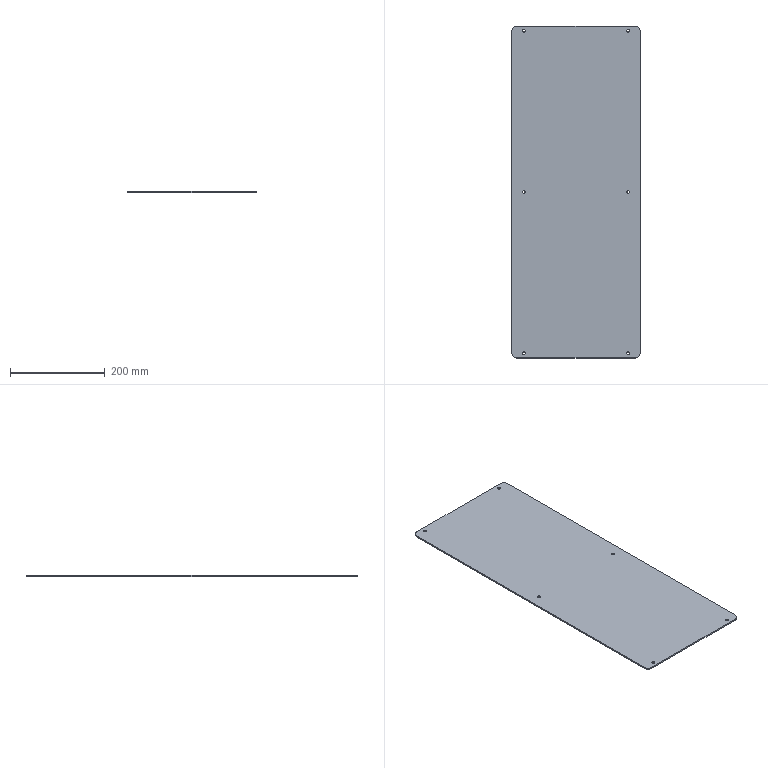Part | STEP file | 09-13 light-transmitting plate | 1 solid | 22 faces | box 270 x 700 x 3 mm | volume 566234 mm3 | cylinder 16 | plane 6 | commonest cylinder face diameters 6 x12 20 x4
STEP:
#1=CARTESIAN_POINT('',(107.,-340.,3.));
#2=VERTEX_POINT('',#1);
#3=CARTESIAN_POINT('',(113.,-340.,3.));
#4=VERTEX_POINT('',#3);
#5=CARTESIAN_POINT('',(110.,-340.,3.));
#6=DIRECTION('',(0.,0.,1.));
#7=DIRECTION('',(1.,0.,0.));
#8=AXIS2_PLACEMENT_3D('',#5,#6,#7);
#9=CIRCLE('',#8,3.);
#10=EDGE_CURVE('',#2,#4,#9,.T.);
#11=ORIENTED_EDGE('',*,*,#10,.T.);
#12=CARTESIAN_POINT('',(113.,-340.,0.));
#13=VERTEX_POINT('',#12);
#14=CARTESIAN_POINT('',(113.,-340.,6.));
#15=DIRECTION('',(0.,0.,-1.));
#16=VECTOR('',#15,1000.);
#17=LINE('',#14,#16);
#18=EDGE_CURVE('',#4,#13,#17,.T.);
#19=ORIENTED_EDGE('',*,*,#18,.T.);
#20=CARTESIAN_POINT('',(107.,-340.,0.));
#21=VERTEX_POINT('',#20);
#22=CARTESIAN_POINT('',(110.,-340.,0.));
#23=DIRECTION('',(0.,0.,-1.));
#24=DIRECTION('',(-1.,0.,0.));
#25=AXIS2_PLACEMENT_3D('',#22,#23,#24);
#26=CIRCLE('',#25,3.);
#27=EDGE_CURVE('',#13,#21,#26,.T.);
#28=ORIENTED_EDGE('',*,*,#27,.T.);
#29=CARTESIAN_POINT('',(107.,-340.,6.));
#30=DIRECTION('',(0.,0.,-1.));
#31=VECTOR('',#30,1000.);
#32=LINE('',#29,#31);
#33=EDGE_CURVE('',#2,#21,#32,.T.);
#34=ORIENTED_EDGE('',*,*,#33,.F.);
#35=EDGE_LOOP('',(#11,#19,#28,#34));
#36=FACE_OUTER_BOUND('',#35,.T.);
#37=CARTESIAN_POINT('',(110.,-340.,6.));
#38=DIRECTION('',(0.,0.,-1.));
#39=DIRECTION('',(-1.,0.,0.));
#40=AXIS2_PLACEMENT_3D('',#37,#38,#39);
#41=CYLINDRICAL_SURFACE('',#40,3.);
#42=ADVANCED_FACE('',(#36),#41,.F.);
#43=CARTESIAN_POINT('',(107.,0.,3.));
#44=VERTEX_POINT('',#43);
#45=CARTESIAN_POINT('',(113.,0.,3.));
#46=VERTEX_POINT('',#45);
#47=CARTESIAN_POINT('',(110.,0.,3.));
#48=DIRECTION('',(0.,0.,1.));
#49=DIRECTION('',(1.,0.,0.));
#50=AXIS2_PLACEMENT_3D('',#47,#48,#49);
#51=CIRCLE('',#50,3.);
#52=EDGE_CURVE('',#44,#46,#51,.T.);
#53=ORIENTED_EDGE('',*,*,#52,.T.);
#54=CARTESIAN_POINT('',(113.,0.,0.));
#55=VERTEX_POINT('',#54);
#56=CARTESIAN_POINT('',(113.,0.,6.));
#57=DIRECTION('',(0.,0.,-1.));
#58=VECTOR('',#57,1000.);
#59=LINE('',#56,#58);
#60=EDGE_CURVE('',#46,#55,#59,.T.);
#61=ORIENTED_EDGE('',*,*,#60,.T.);
#62=CARTESIAN_POINT('',(107.,0.,0.));
#63=VERTEX_POINT('',#62);
#64=CARTESIAN_POINT('',(110.,0.,0.));
#65=DIRECTION('',(0.,0.,-1.));
#66=DIRECTION('',(-1.,0.,0.));
#67=AXIS2_PLACEMENT_3D('',#64,#65,#66);
#68=CIRCLE('',#67,3.);
#69=EDGE_CURVE('',#55,#63,#68,.T.);
#70=ORIENTED_EDGE('',*,*,#69,.T.);
#71=CARTESIAN_POINT('',(107.,0.,6.));
#72=DIRECTION('',(0.,0.,-1.));
#73=VECTOR('',#72,1000.);
#74=LINE('',#71,#73);
#75=EDGE_CURVE('',#44,#63,#74,.T.);
#76=ORIENTED_EDGE('',*,*,#75,.F.);
#77=EDGE_LOOP('',(#53,#61,#70,#76));
#78=FACE_OUTER_BOUND('',#77,.T.);
#79=CARTESIAN_POINT('',(110.,0.,6.));
#80=DIRECTION('',(0.,0.,-1.));
#81=DIRECTION('',(-1.,0.,0.));
#82=AXIS2_PLACEMENT_3D('',#79,#80,#81);
#83=CYLINDRICAL_SURFACE('',#82,3.);
#84=ADVANCED_FACE('',(#78),#83,.F.);
#85=CARTESIAN_POINT('',(-113.,-340.,3.));
#86=VERTEX_POINT('',#85);
#87=CARTESIAN_POINT('',(-107.,-340.,3.));
#88=VERTEX_POINT('',#87);
#89=CARTESIAN_POINT('',(-110.,-340.,3.));
#90=DIRECTION('',(0.,0.,1.));
#91=DIRECTION('',(1.,0.,0.));
#92=AXIS2_PLACEMENT_3D('',#89,#90,#91);
#93=CIRCLE('',#92,3.);
#94=EDGE_CURVE('',#86,#88,#93,.T.);
#95=ORIENTED_EDGE('',*,*,#94,.T.);
#96=CARTESIAN_POINT('',(-107.,-340.,0.));
#97=VERTEX_POINT('',#96);
#98=CARTESIAN_POINT('',(-107.,-340.,6.));
#99=DIRECTION('',(0.,0.,-1.));
#100=VECTOR('',#99,1000.);
#101=LINE('',#98,#100);
#102=EDGE_CURVE('',#88,#97,#101,.T.);
#103=ORIENTED_EDGE('',*,*,#102,.T.);
#104=CARTESIAN_POINT('',(-113.,-340.,0.));
#105=VERTEX_POINT('',#104);
#106=CARTESIAN_POINT('',(-110.,-340.,0.));
#107=DIRECTION('',(0.,0.,-1.));
#108=DIRECTION('',(-1.,0.,0.));
#109=AXIS2_PLACEMENT_3D('',#106,#107,#108);
#110=CIRCLE('',#109,3.);
#111=EDGE_CURVE('',#97,#105,#110,.T.);
#112=ORIENTED_EDGE('',*,*,#111,.T.);
#113=CARTESIAN_POINT('',(-113.,-340.,6.));
#114=DIRECTION('',(0.,0.,-1.));
#115=VECTOR('',#114,1000.);
#116=LINE('',#113,#115);
#117=EDGE_CURVE('',#86,#105,#116,.T.);
#118=ORIENTED_EDGE('',*,*,#117,.F.);
#119=EDGE_LOOP('',(#95,#103,#112,#118));
#120=FACE_OUTER_BOUND('',#119,.T.);
#121=CARTESIAN_POINT('',(-110.,-340.,6.));
#122=DIRECTION('',(0.,0.,-1.));
#123=DIRECTION('',(-1.,0.,0.));
#124=AXIS2_PLACEMENT_3D('',#121,#122,#123);
#125=CYLINDRICAL_SURFACE('',#124,3.);
#126=ADVANCED_FACE('',(#120),#125,.F.);
#127=CARTESIAN_POINT('',(-113.,0.,3.));
#128=VERTEX_POINT('',#127);
#129=CARTESIAN_POINT('',(-107.,0.,3.));
#130=VERTEX_POINT('',#129);
#131=CARTESIAN_POINT('',(-110.,0.,3.));
#132=DIRECTION('',(0.,0.,1.));
#133=DIRECTION('',(1.,0.,0.));
#134=AXIS2_PLACEMENT_3D('',#131,#132,#133);
#135=CIRCLE('',#134,3.);
#136=EDGE_CURVE('',#128,#130,#135,.T.);
#137=ORIENTED_EDGE('',*,*,#136,.T.);
#138=CARTESIAN_POINT('',(-107.,0.,0.));
#139=VERTEX_POINT('',#138);
#140=CARTESIAN_POINT('',(-107.,0.,6.));
#141=DIRECTION('',(0.,0.,-1.));
#142=VECTOR('',#141,1000.);
#143=LINE('',#140,#142);
#144=EDGE_CURVE('',#130,#139,#143,.T.);
#145=ORIENTED_EDGE('',*,*,#144,.T.);
#146=CARTESIAN_POINT('',(-113.,0.,0.));
#147=VERTEX_POINT('',#146);
#148=CARTESIAN_POINT('',(-110.,0.,0.));
#149=DIRECTION('',(0.,0.,-1.));
#150=DIRECTION('',(-1.,0.,0.));
#151=AXIS2_PLACEMENT_3D('',#148,#149,#150);
#152=CIRCLE('',#151,3.);
#153=EDGE_CURVE('',#139,#147,#152,.T.);
#154=ORIENTED_EDGE('',*,*,#153,.T.);
#155=CARTESIAN_POINT('',(-113.,0.,6.));
#156=DIRECTION('',(0.,0.,-1.));
#157=VECTOR('',#156,1000.);
#158=LINE('',#155,#157);
#159=EDGE_CURVE('',#128,#147,#158,.T.);
#160=ORIENTED_EDGE('',*,*,#159,.F.);
#161=EDGE_LOOP('',(#137,#145,#154,#160));
#162=FACE_OUTER_BOUND('',#161,.T.);
#163=CARTESIAN_POINT('',(-110.,0.,6.));
#164=DIRECTION('',(0.,0.,-1.));
#165=DIRECTION('',(-1.,0.,0.));
#166=AXIS2_PLACEMENT_3D('',#163,#164,#165);
#167=CYLINDRICAL_SURFACE('',#166,3.);
#168=ADVANCED_FACE('',(#162),#167,.F.);
#169=CARTESIAN_POINT('',(-113.,340.,3.));
#170=VERTEX_POINT('',#169);
#171=CARTESIAN_POINT('',(-107.,340.,3.));
#172=VERTEX_POINT('',#171);
#173=CARTESIAN_POINT('',(-110.,340.,3.));
#174=DIRECTION('',(0.,0.,1.));
#175=DIRECTION('',(1.,0.,0.));
#176=AXIS2_PLACEMENT_3D('',#173,#174,#175);
#177=CIRCLE('',#176,3.);
#178=EDGE_CURVE('',#170,#172,#177,.T.);
#179=ORIENTED_EDGE('',*,*,#178,.T.);
#180=CARTESIAN_POINT('',(-107.,340.,0.));
#181=VERTEX_POINT('',#180);
#182=CARTESIAN_POINT('',(-107.,340.,6.));
#183=DIRECTION('',(0.,0.,-1.));
#184=VECTOR('',#183,1000.);
#185=LINE('',#182,#184);
#186=EDGE_CURVE('',#172,#181,#185,.T.);
#187=ORIENTED_EDGE('',*,*,#186,.T.);
#188=CARTESIAN_POINT('',(-113.,340.,0.));
#189=VERTEX_POINT('',#188);
#190=CARTESIAN_POINT('',(-110.,340.,0.));
#191=DIRECTION('',(0.,0.,-1.));
#192=DIRECTION('',(-1.,0.,0.));
#193=AXIS2_PLACEMENT_3D('',#190,#191,#192);
#194=CIRCLE('',#193,3.);
#195=EDGE_CURVE('',#181,#189,#194,.T.);
#196=ORIENTED_EDGE('',*,*,#195,.T.);
#197=CARTESIAN_POINT('',(-113.,340.,6.));
#198=DIRECTION('',(0.,0.,-1.));
#199=VECTOR('',#198,1000.);
#200=LINE('',#197,#199);
#201=EDGE_CURVE('',#170,#189,#200,.T.);
#202=ORIENTED_EDGE('',*,*,#201,.F.);
#203=EDGE_LOOP('',(#179,#187,#196,#202));
#204=FACE_OUTER_BOUND('',#203,.T.);
#205=CARTESIAN_POINT('',(-110.,340.,6.));
#206=DIRECTION('',(0.,0.,-1.));
#207=DIRECTION('',(-1.,0.,0.));
#208=AXIS2_PLACEMENT_3D('',#205,#206,#207);
#209=CYLINDRICAL_SURFACE('',#208,3.);
#210=ADVANCED_FACE('',(#204),#209,.F.);
#211=CARTESIAN_POINT('',(107.,340.,3.));
#212=VERTEX_POINT('',#211);
#213=CARTESIAN_POINT('',(113.,340.,3.));
#214=VERTEX_POINT('',#213);
#215=CARTESIAN_POINT('',(110.,340.,3.));
#216=DIRECTION('',(0.,0.,1.));
#217=DIRECTION('',(1.,0.,0.));
#218=AXIS2_PLACEMENT_3D('',#215,#216,#217);
#219=CIRCLE('',#218,3.);
#220=EDGE_CURVE('',#212,#214,#219,.T.);
#221=ORIENTED_EDGE('',*,*,#220,.T.);
#222=CARTESIAN_POINT('',(113.,340.,0.));
#223=VERTEX_POINT('',#222);
#224=CARTESIAN_POINT('',(113.,340.,6.));
#225=DIRECTION('',(0.,0.,-1.));
#226=VECTOR('',#225,1000.);
#227=LINE('',#224,#226);
#228=EDGE_CURVE('',#214,#223,#227,.T.);
#229=ORIENTED_EDGE('',*,*,#228,.T.);
#230=CARTESIAN_POINT('',(107.,340.,0.));
#231=VERTEX_POINT('',#230);
#232=CARTESIAN_POINT('',(110.,340.,0.));
#233=DIRECTION('',(0.,0.,-1.));
#234=DIRECTION('',(-1.,0.,0.));
#235=AXIS2_PLACEMENT_3D('',#232,#233,#234);
#236=CIRCLE('',#235,3.);
#237=EDGE_CURVE('',#223,#231,#236,.T.);
#238=ORIENTED_EDGE('',*,*,#237,.T.);
#239=CARTESIAN_POINT('',(107.,340.,6.));
#240=DIRECTION('',(0.,0.,-1.));
#241=VECTOR('',#240,1000.);
#242=LINE('',#239,#241);
#243=EDGE_CURVE('',#212,#231,#242,.T.);
#244=ORIENTED_EDGE('',*,*,#243,.F.);
#245=EDGE_LOOP('',(#221,#229,#238,#244));
#246=FACE_OUTER_BOUND('',#245,.T.);
#247=CARTESIAN_POINT('',(110.,340.,6.));
#248=DIRECTION('',(0.,0.,-1.));
#249=DIRECTION('',(-1.,0.,0.));
#250=AXIS2_PLACEMENT_3D('',#247,#248,#249);
#251=CYLINDRICAL_SURFACE('',#250,3.);
#252=ADVANCED_FACE('',(#246),#251,.F.);
#253=CARTESIAN_POINT('',(135.,-340.,3.));
#254=VERTEX_POINT('',#253);
#255=CARTESIAN_POINT('',(135.,340.,3.));
#256=VERTEX_POINT('',#255);
#257=CARTESIAN_POINT('',(135.,350.,3.));
#258=DIRECTION('',(0.,1.,0.));
#259=VECTOR('',#258,1000.);
#260=LINE('',#257,#259);
#261=EDGE_CURVE('',#254,#256,#260,.T.);
#262=ORIENTED_EDGE('',*,*,#261,.F.);
#263=CARTESIAN_POINT('',(135.,-340.,0.));
#264=VERTEX_POINT('',#263);
#265=CARTESIAN_POINT('',(135.,-340.,3.));
#266=DIRECTION('',(0.,0.,-1.));
#267=VECTOR('',#266,1000.);
#268=LINE('',#265,#267);
#269=EDGE_CURVE('',#254,#264,#268,.T.);
#270=ORIENTED_EDGE('',*,*,#269,.T.);
#271=CARTESIAN_POINT('',(135.,340.,0.));
#272=VERTEX_POINT('',#271);
#273=CARTESIAN_POINT('',(135.,350.,0.));
#274=DIRECTION('',(0.,1.,0.));
#275=VECTOR('',#274,1000.);
#276=LINE('',#273,#275);
#277=EDGE_CURVE('',#264,#272,#276,.T.);
#278=ORIENTED_EDGE('',*,*,#277,.T.);
#279=CARTESIAN_POINT('',(135.,340.,3.));
#280=DIRECTION('',(0.,0.,1.));
#281=VECTOR('',#280,1000.);
#282=LINE('',#279,#281);
#283=EDGE_CURVE('',#272,#256,#282,.T.);
#284=ORIENTED_EDGE('',*,*,#283,.T.);
#285=EDGE_LOOP('',(#262,#270,#278,#284));
#286=FACE_OUTER_BOUND('',#285,.T.);
#287=CARTESIAN_POINT('',(135.,350.,3.));
#288=DIRECTION('',(-1.,0.,0.));
#289=DIRECTION('',(0.,-1.,0.));
#290=AXIS2_PLACEMENT_3D('',#287,#288,#289);
#291=PLANE('',#290);
#292=ADVANCED_FACE('',(#286),#291,.F.);
#293=CARTESIAN_POINT('',(125.,350.,0.));
#294=VERTEX_POINT('',#293);
#295=CARTESIAN_POINT('',(-125.,350.,0.));
#296=VERTEX_POINT('',#295);
#297=CARTESIAN_POINT('',(-135.,350.,0.));
#298=DIRECTION('',(-1.,0.,0.));
#299=VECTOR('',#298,1000.);
#300=LINE('',#297,#299);
#301=EDGE_CURVE('',#294,#296,#300,.T.);
#302=ORIENTED_EDGE('',*,*,#301,.T.);
#303=CARTESIAN_POINT('',(-125.,350.,3.));
#304=VERTEX_POINT('',#303);
#305=CARTESIAN_POINT('',(-125.,350.,3.));
#306=DIRECTION('',(0.,0.,1.));
#307=VECTOR('',#306,1000.);
#308=LINE('',#305,#307);
#309=EDGE_CURVE('',#296,#304,#308,.T.);
#310=ORIENTED_EDGE('',*,*,#309,.T.);
#311=CARTESIAN_POINT('',(125.,350.,3.));
#312=VERTEX_POINT('',#311);
#313=CARTESIAN_POINT('',(-135.,350.,3.));
#314=DIRECTION('',(-1.,0.,0.));
#315=VECTOR('',#314,1000.);
#316=LINE('',#313,#315);
#317=EDGE_CURVE('',#312,#304,#316,.T.);
#318=ORIENTED_EDGE('',*,*,#317,.F.);
#319=CARTESIAN_POINT('',(125.,350.,3.));
#320=DIRECTION('',(0.,0.,-1.));
#321=VECTOR('',#320,1000.);
#322=LINE('',#319,#321);
#323=EDGE_CURVE('',#312,#294,#322,.T.);
#324=ORIENTED_EDGE('',*,*,#323,.T.);
#325=EDGE_LOOP('',(#302,#310,#318,#324));
#326=FACE_OUTER_BOUND('',#325,.T.);
#327=CARTESIAN_POINT('',(-135.,350.,3.));
#328=DIRECTION('',(0.,-1.,0.));
#329=DIRECTION('',(0.,0.,-1.));
#330=AXIS2_PLACEMENT_3D('',#327,#328,#329);
#331=PLANE('',#330);
#332=ADVANCED_FACE('',(#326),#331,.F.);
#333=CARTESIAN_POINT('',(-135.,340.,0.));
#334=VERTEX_POINT('',#333);
#335=CARTESIAN_POINT('',(-135.,-340.,0.));
#336=VERTEX_POINT('',#335);
#337=CARTESIAN_POINT('',(-135.,350.,0.));
#338=DIRECTION('',(0.,-1.,0.));
#339=VECTOR('',#338,1000.);
#340=LINE('',#337,#339);
#341=EDGE_CURVE('',#334,#336,#340,.T.);
#342=ORIENTED_EDGE('',*,*,#341,.T.);
#343=CARTESIAN_POINT('',(-135.,-340.,3.));
#344=VERTEX_POINT('',#343);
#345=CARTESIAN_POINT('',(-135.,-340.,3.));
#346=DIRECTION('',(0.,0.,1.));
#347=VECTOR('',#346,1000.);
#348=LINE('',#345,#347);
#349=EDGE_CURVE('',#336,#344,#348,.T.);
#350=ORIENTED_EDGE('',*,*,#349,.T.);
#351=CARTESIAN_POINT('',(-135.,340.,3.));
#352=VERTEX_POINT('',#351);
#353=CARTESIAN_POINT('',(-135.,350.,3.));
#354=DIRECTION('',(0.,-1.,0.));
#355=VECTOR('',#354,1000.);
#356=LINE('',#353,#355);
#357=EDGE_CURVE('',#352,#344,#356,.T.);
#358=ORIENTED_EDGE('',*,*,#357,.F.);
#359=CARTESIAN_POINT('',(-135.,340.,3.));
#360=DIRECTION('',(0.,0.,-1.));
#361=VECTOR('',#360,1000.);
#362=LINE('',#359,#361);
#363=EDGE_CURVE('',#352,#334,#362,.T.);
#364=ORIENTED_EDGE('',*,*,#363,.T.);
#365=EDGE_LOOP('',(#342,#350,#358,#364));
#366=FACE_OUTER_BOUND('',#365,.T.);
#367=CARTESIAN_POINT('',(-135.,350.,3.));
#368=DIRECTION('',(1.,0.,0.));
#369=DIRECTION('',(0.,1.,0.));
#370=AXIS2_PLACEMENT_3D('',#367,#368,#369);
#371=PLANE('',#370);
#372=ADVANCED_FACE('',(#366),#371,.F.);
#373=CARTESIAN_POINT('',(-125.,-350.,0.));
#374=VERTEX_POINT('',#373);
#375=CARTESIAN_POINT('',(125.,-350.,0.));
#376=VERTEX_POINT('',#375);
#377=CARTESIAN_POINT('',(-135.,-350.,0.));
#378=DIRECTION('',(1.,0.,0.));
#379=VECTOR('',#378,1000.);
#380=LINE('',#377,#379);
#381=EDGE_CURVE('',#374,#376,#380,.T.);
#382=ORIENTED_EDGE('',*,*,#381,.T.);
#383=CARTESIAN_POINT('',(125.,-350.,3.));
#384=VERTEX_POINT('',#383);
#385=CARTESIAN_POINT('',(125.,-350.,3.));
#386=DIRECTION('',(0.,0.,1.));
#387=VECTOR('',#386,1000.);
#388=LINE('',#385,#387);
#389=EDGE_CURVE('',#376,#384,#388,.T.);
#390=ORIENTED_EDGE('',*,*,#389,.T.);
#391=CARTESIAN_POINT('',(-125.,-350.,3.));
#392=VERTEX_POINT('',#391);
#393=CARTESIAN_POINT('',(-135.,-350.,3.));
#394=DIRECTION('',(1.,0.,0.));
#395=VECTOR('',#394,1000.);
#396=LINE('',#393,#395);
#397=EDGE_CURVE('',#392,#384,#396,.T.);
#398=ORIENTED_EDGE('',*,*,#397,.F.);
#399=CARTESIAN_POINT('',(-125.,-350.,3.));
#400=DIRECTION('',(0.,0.,-1.));
#401=VECTOR('',#400,1000.);
#402=LINE('',#399,#401);
#403=EDGE_CURVE('',#392,#374,#402,.T.);
#404=ORIENTED_EDGE('',*,*,#403,.T.);
#405=EDGE_LOOP('',(#382,#390,#398,#404));
#406=FACE_OUTER_BOUND('',#405,.T.);
#407=CARTESIAN_POINT('',(-135.,-350.,3.));
#408=DIRECTION('',(0.,1.,0.));
#409=DIRECTION('',(0.,0.,1.));
#410=AXIS2_PLACEMENT_3D('',#407,#408,#409);
#411=PLANE('',#410);
#412=ADVANCED_FACE('',(#406),#411,.F.);
#413=ORIENTED_EDGE('',*,*,#52,.F.);
#414=CARTESIAN_POINT('',(110.,0.,3.));
#415=DIRECTION('',(0.,0.,1.));
#416=DIRECTION('',(1.,0.,0.));
#417=AXIS2_PLACEMENT_3D('',#414,#415,#416);
#418=CIRCLE('',#417,3.);
#419=EDGE_CURVE('',#46,#44,#418,.T.);
#420=ORIENTED_EDGE('',*,*,#419,.F.);
#421=EDGE_LOOP('',(#413,#420));
#422=FACE_BOUND('',#421,.T.);
#423=ORIENTED_EDGE('',*,*,#136,.F.);
#424=CARTESIAN_POINT('',(-110.,0.,3.));
#425=DIRECTION('',(0.,0.,1.));
#426=DIRECTION('',(1.,0.,0.));
#427=AXIS2_PLACEMENT_3D('',#424,#425,#426);
#428=CIRCLE('',#427,3.);
#429=EDGE_CURVE('',#130,#128,#428,.T.);
#430=ORIENTED_EDGE('',*,*,#429,.F.);
#431=EDGE_LOOP('',(#423,#430));
#432=FACE_BOUND('',#431,.T.);
#433=ORIENTED_EDGE('',*,*,#178,.F.);
#434=CARTESIAN_POINT('',(-110.,340.,3.));
#435=DIRECTION('',(0.,0.,1.));
#436=DIRECTION('',(1.,0.,0.));
#437=AXIS2_PLACEMENT_3D('',#434,#435,#436);
#438=CIRCLE('',#437,3.);
#439=EDGE_CURVE('',#172,#170,#438,.T.);
#440=ORIENTED_EDGE('',*,*,#439,.F.);
#441=EDGE_LOOP('',(#433,#440));
#442=FACE_BOUND('',#441,.T.);
#443=ORIENTED_EDGE('',*,*,#220,.F.);
#444=CARTESIAN_POINT('',(110.,340.,3.));
#445=DIRECTION('',(0.,0.,1.));
#446=DIRECTION('',(1.,0.,0.));
#447=AXIS2_PLACEMENT_3D('',#444,#445,#446);
#448=CIRCLE('',#447,3.);
#449=EDGE_CURVE('',#214,#212,#448,.T.);
#450=ORIENTED_EDGE('',*,*,#449,.F.);
#451=EDGE_LOOP('',(#443,#450));
#452=FACE_BOUND('',#451,.T.);
#453=ORIENTED_EDGE('',*,*,#397,.T.);
#454=CARTESIAN_POINT('',(125.,-340.,3.));
#455=DIRECTION('',(0.,0.,1.));
#456=DIRECTION('',(1.,0.,0.));
#457=AXIS2_PLACEMENT_3D('',#454,#455,#456);
#458=CIRCLE('',#457,10.);
#459=EDGE_CURVE('',#384,#254,#458,.T.);
#460=ORIENTED_EDGE('',*,*,#459,.T.);
#461=ORIENTED_EDGE('',*,*,#261,.T.);
#462=CARTESIAN_POINT('',(125.,340.,3.));
#463=DIRECTION('',(0.,0.,1.));
#464=DIRECTION('',(1.,0.,0.));
#465=AXIS2_PLACEMENT_3D('',#462,#463,#464);
#466=CIRCLE('',#465,10.);
#467=EDGE_CURVE('',#256,#312,#466,.T.);
#468=ORIENTED_EDGE('',*,*,#467,.T.);
#469=ORIENTED_EDGE('',*,*,#317,.T.);
#470=CARTESIAN_POINT('',(-125.,340.,3.));
#471=DIRECTION('',(0.,0.,1.));
#472=DIRECTION('',(1.,0.,0.));
#473=AXIS2_PLACEMENT_3D('',#470,#471,#472);
#474=CIRCLE('',#473,10.);
#475=EDGE_CURVE('',#304,#352,#474,.T.);
#476=ORIENTED_EDGE('',*,*,#475,.T.);
#477=ORIENTED_EDGE('',*,*,#357,.T.);
#478=CARTESIAN_POINT('',(-125.,-340.,3.));
#479=DIRECTION('',(0.,0.,1.));
#480=DIRECTION('',(1.,0.,0.));
#481=AXIS2_PLACEMENT_3D('',#478,#479,#480);
#482=CIRCLE('',#481,10.);
#483=EDGE_CURVE('',#344,#392,#482,.T.);
#484=ORIENTED_EDGE('',*,*,#483,.T.);
#485=EDGE_LOOP('',(#453,#460,#461,#468,#469,#476,#477,#484));
#486=FACE_OUTER_BOUND('',#485,.T.);
#487=ORIENTED_EDGE('',*,*,#94,.F.);
#488=CARTESIAN_POINT('',(-110.,-340.,3.));
#489=DIRECTION('',(0.,0.,1.));
#490=DIRECTION('',(1.,0.,0.));
#491=AXIS2_PLACEMENT_3D('',#488,#489,#490);
#492=CIRCLE('',#491,3.);
#493=EDGE_CURVE('',#88,#86,#492,.T.);
#494=ORIENTED_EDGE('',*,*,#493,.F.);
#495=EDGE_LOOP('',(#487,#494));
#496=FACE_BOUND('',#495,.T.);
#497=ORIENTED_EDGE('',*,*,#10,.F.);
#498=CARTESIAN_POINT('',(110.,-340.,3.));
#499=DIRECTION('',(0.,0.,1.));
#500=DIRECTION('',(1.,0.,0.));
#501=AXIS2_PLACEMENT_3D('',#498,#499,#500);
#502=CIRCLE('',#501,3.);
#503=EDGE_CURVE('',#4,#2,#502,.T.);
#504=ORIENTED_EDGE('',*,*,#503,.F.);
#505=EDGE_LOOP('',(#497,#504));
#506=FACE_BOUND('',#505,.T.);
#507=CARTESIAN_POINT('',(135.,-350.,3.));
#508=DIRECTION('',(0.,0.,1.));
#509=DIRECTION('',(1.,0.,0.));
#510=AXIS2_PLACEMENT_3D('',#507,#508,#509);
#511=PLANE('',#510);
#512=ADVANCED_FACE('',(#422,#432,#442,#452,#486,#496,#506),#511,.T.);
#513=CARTESIAN_POINT('',(110.,0.,0.));
#514=DIRECTION('',(0.,0.,-1.));
#515=DIRECTION('',(-1.,0.,0.));
#516=AXIS2_PLACEMENT_3D('',#513,#514,#515);
#517=CIRCLE('',#516,3.);
#518=EDGE_CURVE('',#63,#55,#517,.T.);
#519=ORIENTED_EDGE('',*,*,#518,.F.);
#520=ORIENTED_EDGE('',*,*,#69,.F.);
#521=EDGE_LOOP('',(#519,#520));
#522=FACE_BOUND('',#521,.T.);
#523=CARTESIAN_POINT('',(-110.,0.,0.));
#524=DIRECTION('',(0.,0.,-1.));
#525=DIRECTION('',(-1.,0.,0.));
#526=AXIS2_PLACEMENT_3D('',#523,#524,#525);
#527=CIRCLE('',#526,3.);
#528=EDGE_CURVE('',#147,#139,#527,.T.);
#529=ORIENTED_EDGE('',*,*,#528,.F.);
#530=ORIENTED_EDGE('',*,*,#153,.F.);
#531=EDGE_LOOP('',(#529,#530));
#532=FACE_BOUND('',#531,.T.);
#533=CARTESIAN_POINT('',(-110.,340.,0.));
#534=DIRECTION('',(0.,0.,-1.));
#535=DIRECTION('',(-1.,0.,0.));
#536=AXIS2_PLACEMENT_3D('',#533,#534,#535);
#537=CIRCLE('',#536,3.);
#538=EDGE_CURVE('',#189,#181,#537,.T.);
#539=ORIENTED_EDGE('',*,*,#538,.F.);
#540=ORIENTED_EDGE('',*,*,#195,.F.);
#541=EDGE_LOOP('',(#539,#540));
#542=FACE_BOUND('',#541,.T.);
#543=CARTESIAN_POINT('',(110.,340.,0.));
#544=DIRECTION('',(0.,0.,-1.));
#545=DIRECTION('',(-1.,0.,0.));
#546=AXIS2_PLACEMENT_3D('',#543,#544,#545);
#547=CIRCLE('',#546,3.);
#548=EDGE_CURVE('',#231,#223,#547,.T.);
#549=ORIENTED_EDGE('',*,*,#548,.F.);
#550=ORIENTED_EDGE('',*,*,#237,.F.);
#551=EDGE_LOOP('',(#549,#550));
#552=FACE_BOUND('',#551,.T.);
#553=ORIENTED_EDGE('',*,*,#277,.F.);
#554=CARTESIAN_POINT('',(125.,-340.,0.));
#555=DIRECTION('',(0.,0.,-1.));
#556=DIRECTION('',(1.,0.,0.));
#557=AXIS2_PLACEMENT_3D('',#554,#555,#556);
#558=CIRCLE('',#557,10.);
#559=EDGE_CURVE('',#264,#376,#558,.T.);
#560=ORIENTED_EDGE('',*,*,#559,.T.);
#561=ORIENTED_EDGE('',*,*,#381,.F.);
#562=CARTESIAN_POINT('',(-125.,-340.,0.));
#563=DIRECTION('',(0.,0.,-1.));
#564=DIRECTION('',(1.,0.,0.));
#565=AXIS2_PLACEMENT_3D('',#562,#563,#564);
#566=CIRCLE('',#565,10.);
#567=EDGE_CURVE('',#374,#336,#566,.T.);
#568=ORIENTED_EDGE('',*,*,#567,.T.);
#569=ORIENTED_EDGE('',*,*,#341,.F.);
#570=CARTESIAN_POINT('',(-125.,340.,0.));
#571=DIRECTION('',(0.,0.,-1.));
#572=DIRECTION('',(1.,0.,0.));
#573=AXIS2_PLACEMENT_3D('',#570,#571,#572);
#574=CIRCLE('',#573,10.);
#575=EDGE_CURVE('',#334,#296,#574,.T.);
#576=ORIENTED_EDGE('',*,*,#575,.T.);
#577=ORIENTED_EDGE('',*,*,#301,.F.);
#578=CARTESIAN_POINT('',(125.,340.,0.));
#579=DIRECTION('',(0.,0.,-1.));
#580=DIRECTION('',(1.,0.,0.));
#581=AXIS2_PLACEMENT_3D('',#578,#579,#580);
#582=CIRCLE('',#581,10.);
#583=EDGE_CURVE('',#294,#272,#582,.T.);
#584=ORIENTED_EDGE('',*,*,#583,.T.);
#585=EDGE_LOOP('',(#553,#560,#561,#568,#569,#576,#577,#584));
#586=FACE_OUTER_BOUND('',#585,.T.);
#587=CARTESIAN_POINT('',(-110.,-340.,0.));
#588=DIRECTION('',(0.,0.,-1.));
#589=DIRECTION('',(-1.,0.,0.));
#590=AXIS2_PLACEMENT_3D('',#587,#588,#589);
#591=CIRCLE('',#590,3.);
#592=EDGE_CURVE('',#105,#97,#591,.T.);
#593=ORIENTED_EDGE('',*,*,#592,.F.);
#594=ORIENTED_EDGE('',*,*,#111,.F.);
#595=EDGE_LOOP('',(#593,#594));
#596=FACE_BOUND('',#595,.T.);
#597=CARTESIAN_POINT('',(110.,-340.,0.));
#598=DIRECTION('',(0.,0.,-1.));
#599=DIRECTION('',(-1.,0.,0.));
#600=AXIS2_PLACEMENT_3D('',#597,#598,#599);
#601=CIRCLE('',#600,3.);
#602=EDGE_CURVE('',#21,#13,#601,.T.);
#603=ORIENTED_EDGE('',*,*,#602,.F.);
#604=ORIENTED_EDGE('',*,*,#27,.F.);
#605=EDGE_LOOP('',(#603,#604));
#606=FACE_BOUND('',#605,.T.);
#607=CARTESIAN_POINT('',(135.,-350.,0.));
#608=DIRECTION('',(0.,0.,1.));
#609=DIRECTION('',(1.,0.,0.));
#610=AXIS2_PLACEMENT_3D('',#607,#608,#609);
#611=PLANE('',#610);
#612=ADVANCED_FACE('',(#522,#532,#542,#552,#586,#596,#606),#611,.F.);
#613=ORIENTED_EDGE('',*,*,#228,.F.);
#614=ORIENTED_EDGE('',*,*,#449,.T.);
#615=ORIENTED_EDGE('',*,*,#243,.T.);
#616=ORIENTED_EDGE('',*,*,#548,.T.);
#617=EDGE_LOOP('',(#613,#614,#615,#616));
#618=FACE_OUTER_BOUND('',#617,.T.);
#619=CARTESIAN_POINT('',(110.,340.,6.));
#620=DIRECTION('',(0.,0.,-1.));
#621=DIRECTION('',(-1.,0.,0.));
#622=AXIS2_PLACEMENT_3D('',#619,#620,#621);
#623=CYLINDRICAL_SURFACE('',#622,3.);
#624=ADVANCED_FACE('',(#618),#623,.F.);
#625=ORIENTED_EDGE('',*,*,#186,.F.);
#626=ORIENTED_EDGE('',*,*,#439,.T.);
#627=ORIENTED_EDGE('',*,*,#201,.T.);
#628=ORIENTED_EDGE('',*,*,#538,.T.);
#629=EDGE_LOOP('',(#625,#626,#627,#628));
#630=FACE_OUTER_BOUND('',#629,.T.);
#631=CARTESIAN_POINT('',(-110.,340.,6.));
#632=DIRECTION('',(0.,0.,-1.));
#633=DIRECTION('',(-1.,0.,0.));
#634=AXIS2_PLACEMENT_3D('',#631,#632,#633);
#635=CYLINDRICAL_SURFACE('',#634,3.);
#636=ADVANCED_FACE('',(#630),#635,.F.);
#637=ORIENTED_EDGE('',*,*,#144,.F.);
#638=ORIENTED_EDGE('',*,*,#429,.T.);
#639=ORIENTED_EDGE('',*,*,#159,.T.);
#640=ORIENTED_EDGE('',*,*,#528,.T.);
#641=EDGE_LOOP('',(#637,#638,#639,#640));
#642=FACE_OUTER_BOUND('',#641,.T.);
#643=CARTESIAN_POINT('',(-110.,0.,6.));
#644=DIRECTION('',(0.,0.,-1.));
#645=DIRECTION('',(-1.,0.,0.));
#646=AXIS2_PLACEMENT_3D('',#643,#644,#645);
#647=CYLINDRICAL_SURFACE('',#646,3.);
#648=ADVANCED_FACE('',(#642),#647,.F.);
#649=ORIENTED_EDGE('',*,*,#102,.F.);
#650=ORIENTED_EDGE('',*,*,#493,.T.);
#651=ORIENTED_EDGE('',*,*,#117,.T.);
#652=ORIENTED_EDGE('',*,*,#592,.T.);
#653=EDGE_LOOP('',(#649,#650,#651,#652));
#654=FACE_OUTER_BOUND('',#653,.T.);
#655=CARTESIAN_POINT('',(-110.,-340.,6.));
#656=DIRECTION('',(0.,0.,-1.));
#657=DIRECTION('',(-1.,0.,0.));
#658=AXIS2_PLACEMENT_3D('',#655,#656,#657);
#659=CYLINDRICAL_SURFACE('',#658,3.);
#660=ADVANCED_FACE('',(#654),#659,.F.);
#661=ORIENTED_EDGE('',*,*,#60,.F.);
#662=ORIENTED_EDGE('',*,*,#419,.T.);
#663=ORIENTED_EDGE('',*,*,#75,.T.);
#664=ORIENTED_EDGE('',*,*,#518,.T.);
#665=EDGE_LOOP('',(#661,#662,#663,#664));
#666=FACE_OUTER_BOUND('',#665,.T.);
#667=CARTESIAN_POINT('',(110.,0.,6.));
#668=DIRECTION('',(0.,0.,-1.));
#669=DIRECTION('',(-1.,0.,0.));
#670=AXIS2_PLACEMENT_3D('',#667,#668,#669);
#671=CYLINDRICAL_SURFACE('',#670,3.);
#672=ADVANCED_FACE('',(#666),#671,.F.);
#673=ORIENTED_EDGE('',*,*,#18,.F.);
#674=ORIENTED_EDGE('',*,*,#503,.T.);
#675=ORIENTED_EDGE('',*,*,#33,.T.);
#676=ORIENTED_EDGE('',*,*,#602,.T.);
#677=EDGE_LOOP('',(#673,#674,#675,#676));
#678=FACE_OUTER_BOUND('',#677,.T.);
#679=CARTESIAN_POINT('',(110.,-340.,6.));
#680=DIRECTION('',(0.,0.,-1.));
#681=DIRECTION('',(-1.,0.,0.));
#682=AXIS2_PLACEMENT_3D('',#679,#680,#681);
#683=CYLINDRICAL_SURFACE('',#682,3.);
#684=ADVANCED_FACE('',(#678),#683,.F.);
#685=ORIENTED_EDGE('',*,*,#459,.F.);
#686=ORIENTED_EDGE('',*,*,#389,.F.);
#687=ORIENTED_EDGE('',*,*,#559,.F.);
#688=ORIENTED_EDGE('',*,*,#269,.F.);
#689=EDGE_LOOP('',(#685,#686,#687,#688));
#690=FACE_OUTER_BOUND('',#689,.T.);
#691=CARTESIAN_POINT('',(125.,-340.,3.));
#692=DIRECTION('',(0.,0.,-1.));
#693=DIRECTION('',(-1.,0.,0.));
#694=AXIS2_PLACEMENT_3D('',#691,#692,#693);
#695=CYLINDRICAL_SURFACE('',#694,10.);
#696=ADVANCED_FACE('',(#690),#695,.T.);
#697=ORIENTED_EDGE('',*,*,#483,.F.);
#698=ORIENTED_EDGE('',*,*,#349,.F.);
#699=ORIENTED_EDGE('',*,*,#567,.F.);
#700=ORIENTED_EDGE('',*,*,#403,.F.);
#701=EDGE_LOOP('',(#697,#698,#699,#700));
#702=FACE_OUTER_BOUND('',#701,.T.);
#703=CARTESIAN_POINT('',(-125.,-340.,3.));
#704=DIRECTION('',(0.,0.,-1.));
#705=DIRECTION('',(-1.,0.,0.));
#706=AXIS2_PLACEMENT_3D('',#703,#704,#705);
#707=CYLINDRICAL_SURFACE('',#706,10.);
#708=ADVANCED_FACE('',(#702),#707,.T.);
#709=ORIENTED_EDGE('',*,*,#475,.F.);
#710=ORIENTED_EDGE('',*,*,#309,.F.);
#711=ORIENTED_EDGE('',*,*,#575,.F.);
#712=ORIENTED_EDGE('',*,*,#363,.F.);
#713=EDGE_LOOP('',(#709,#710,#711,#712));
#714=FACE_OUTER_BOUND('',#713,.T.);
#715=CARTESIAN_POINT('',(-125.,340.,3.));
#716=DIRECTION('',(0.,0.,-1.));
#717=DIRECTION('',(-1.,0.,0.));
#718=AXIS2_PLACEMENT_3D('',#715,#716,#717);
#719=CYLINDRICAL_SURFACE('',#718,10.);
#720=ADVANCED_FACE('',(#714),#719,.T.);
#721=ORIENTED_EDGE('',*,*,#467,.F.);
#722=ORIENTED_EDGE('',*,*,#283,.F.);
#723=ORIENTED_EDGE('',*,*,#583,.F.);
#724=ORIENTED_EDGE('',*,*,#323,.F.);
#725=EDGE_LOOP('',(#721,#722,#723,#724));
#726=FACE_OUTER_BOUND('',#725,.T.);
#727=CARTESIAN_POINT('',(125.,340.,3.));
#728=DIRECTION('',(0.,0.,-1.));
#729=DIRECTION('',(-1.,0.,0.));
#730=AXIS2_PLACEMENT_3D('',#727,#728,#729);
#731=CYLINDRICAL_SURFACE('',#730,10.);
#732=ADVANCED_FACE('',(#726),#731,.T.);
#733=CLOSED_SHELL('',(#42,#84,#126,#168,#210,#252,#292,#332,#372,#412,#512,#612,#624,#636,#648,#660,#672,#684,#696,#708,#720,#732));
#734=MANIFOLD_SOLID_BREP('',#733);
#735=CARTESIAN_POINT('',(0.,0.,0.));
#736=DIRECTION('',(0.,0.,1.));
#737=DIRECTION('',(1.,0.,0.));
#738=AXIS2_PLACEMENT_3D('',#735,#736,#737);
#739=(LENGTH_UNIT()NAMED_UNIT(*)SI_UNIT(.MILLI.,.METRE.));
#740=UNCERTAINTY_MEASURE_WITH_UNIT(LENGTH_MEASURE(0.00001),#739,'','');
#741=(NAMED_UNIT(*)PLANE_ANGLE_UNIT()SI_UNIT($,.RADIAN.));
#742=(NAMED_UNIT(*)SI_UNIT($,.STERADIAN.)SOLID_ANGLE_UNIT());
#743=(GEOMETRIC_REPRESENTATION_CONTEXT(3)GLOBAL_UNCERTAINTY_ASSIGNED_CONTEXT((#740))GLOBAL_UNIT_ASSIGNED_CONTEXT((#739,#741,#742))REPRESENTATION_CONTEXT('',''));
#744=ADVANCED_BREP_SHAPE_REPRESENTATION('',(#734,#738),#743);